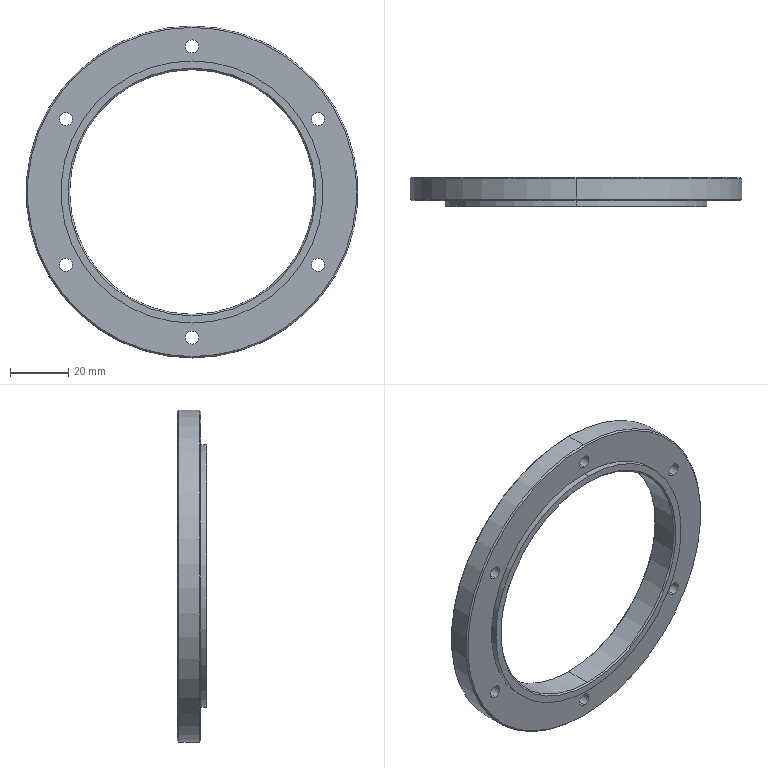Part | STEP file | 10-08 bearing seat cover plate lower | 1 solid | 47 faces | box 114 x 10 x 114 mm | volume 37218 mm3 | cylinder 30 | plane 9 | cone 8 | commonest cylinder face diameters 4.5 x12 8 x12 84 x2 90 x2 114 x2
STEP:
#1=CARTESIAN_POINT('',(0.,-0.5,-42.));
#2=VERTEX_POINT('',#1);
#3=CARTESIAN_POINT('',(0.,-0.5,42.));
#4=VERTEX_POINT('',#3);
#5=CARTESIAN_POINT('',(0.,-0.5,0.));
#6=DIRECTION('',(0.,1.,0.));
#7=DIRECTION('',(0.,0.,-1.));
#8=AXIS2_PLACEMENT_3D('',#5,#6,#7);
#9=CIRCLE('',#8,42.);
#10=EDGE_CURVE('',#2,#4,#9,.T.);
#11=ORIENTED_EDGE('',*,*,#10,.F.);
#12=CARTESIAN_POINT('',(0.,0.,-42.5));
#13=VERTEX_POINT('',#12);
#14=CARTESIAN_POINT('',(0.,-0.5,-42.));
#15=DIRECTION('',(0.,0.7071,-0.7071));
#16=VECTOR('',#15,1000.);
#17=LINE('',#14,#16);
#18=EDGE_CURVE('',#2,#13,#17,.T.);
#19=ORIENTED_EDGE('',*,*,#18,.T.);
#20=CARTESIAN_POINT('',(0.,0.,42.5));
#21=VERTEX_POINT('',#20);
#22=CARTESIAN_POINT('',(0.,0.,0.));
#23=DIRECTION('',(0.,-1.,0.));
#24=DIRECTION('',(0.,0.,-1.));
#25=AXIS2_PLACEMENT_3D('',#22,#23,#24);
#26=CIRCLE('',#25,42.5);
#27=EDGE_CURVE('',#21,#13,#26,.T.);
#28=ORIENTED_EDGE('',*,*,#27,.F.);
#29=CARTESIAN_POINT('',(0.,-0.5,42.));
#30=DIRECTION('',(0.,0.7071,0.7071));
#31=VECTOR('',#30,1000.);
#32=LINE('',#29,#31);
#33=EDGE_CURVE('',#4,#21,#32,.T.);
#34=ORIENTED_EDGE('',*,*,#33,.F.);
#35=EDGE_LOOP('',(#11,#19,#28,#34));
#36=FACE_OUTER_BOUND('',#35,.T.);
#37=CARTESIAN_POINT('',(0.,-0.5,0.));
#38=DIRECTION('',(0.,1.,0.));
#39=DIRECTION('',(0.,0.,1.));
#40=AXIS2_PLACEMENT_3D('',#37,#38,#39);
#41=CONICAL_SURFACE('',#40,42.,0.7854);
#42=ADVANCED_FACE('',(#36),#41,.F.);
#43=CARTESIAN_POINT('',(0.,0.,56.5));
#44=VERTEX_POINT('',#43);
#45=CARTESIAN_POINT('',(0.,0.,-56.5));
#46=VERTEX_POINT('',#45);
#47=CARTESIAN_POINT('',(0.,0.,0.));
#48=DIRECTION('',(0.,1.,0.));
#49=DIRECTION('',(0.,0.,-1.));
#50=AXIS2_PLACEMENT_3D('',#47,#48,#49);
#51=CIRCLE('',#50,56.5);
#52=EDGE_CURVE('',#44,#46,#51,.T.);
#53=ORIENTED_EDGE('',*,*,#52,.F.);
#54=CARTESIAN_POINT('',(0.,-0.5,57.));
#55=VERTEX_POINT('',#54);
#56=CARTESIAN_POINT('',(0.,0.,56.5));
#57=DIRECTION('',(0.,-0.7071,0.7071));
#58=VECTOR('',#57,1000.);
#59=LINE('',#56,#58);
#60=EDGE_CURVE('',#44,#55,#59,.T.);
#61=ORIENTED_EDGE('',*,*,#60,.T.);
#62=CARTESIAN_POINT('',(0.,-0.5,-57.));
#63=VERTEX_POINT('',#62);
#64=CARTESIAN_POINT('',(0.,-0.5,0.));
#65=DIRECTION('',(0.,-1.,0.));
#66=DIRECTION('',(0.,0.,-1.));
#67=AXIS2_PLACEMENT_3D('',#64,#65,#66);
#68=CIRCLE('',#67,57.);
#69=EDGE_CURVE('',#63,#55,#68,.T.);
#70=ORIENTED_EDGE('',*,*,#69,.F.);
#71=CARTESIAN_POINT('',(0.,0.,-56.5));
#72=DIRECTION('',(0.,-0.7071,-0.7071));
#73=VECTOR('',#72,1000.);
#74=LINE('',#71,#73);
#75=EDGE_CURVE('',#46,#63,#74,.T.);
#76=ORIENTED_EDGE('',*,*,#75,.F.);
#77=EDGE_LOOP('',(#53,#61,#70,#76));
#78=FACE_OUTER_BOUND('',#77,.T.);
#79=CARTESIAN_POINT('',(0.,0.,0.));
#80=DIRECTION('',(0.,-1.,0.));
#81=DIRECTION('',(0.,0.,-1.));
#82=AXIS2_PLACEMENT_3D('',#79,#80,#81);
#83=CONICAL_SURFACE('',#82,56.5,0.7854);
#84=ADVANCED_FACE('',(#78),#83,.T.);
#85=CARTESIAN_POINT('',(0.,-9.5,42.));
#86=VERTEX_POINT('',#85);
#87=CARTESIAN_POINT('',(0.,-9.5,-42.));
#88=VERTEX_POINT('',#87);
#89=CARTESIAN_POINT('',(0.,-9.5,0.));
#90=DIRECTION('',(0.,-1.,0.));
#91=DIRECTION('',(0.,0.,1.));
#92=AXIS2_PLACEMENT_3D('',#89,#90,#91);
#93=CIRCLE('',#92,42.);
#94=EDGE_CURVE('',#86,#88,#93,.T.);
#95=ORIENTED_EDGE('',*,*,#94,.F.);
#96=CARTESIAN_POINT('',(0.,-10.,42.5));
#97=VERTEX_POINT('',#96);
#98=CARTESIAN_POINT('',(0.,-10.,42.5));
#99=DIRECTION('',(0.,-0.7071,0.7071));
#100=VECTOR('',#99,1000.);
#101=LINE('',#98,#100);
#102=EDGE_CURVE('',#86,#97,#101,.T.);
#103=ORIENTED_EDGE('',*,*,#102,.T.);
#104=CARTESIAN_POINT('',(0.,-10.,-42.5));
#105=VERTEX_POINT('',#104);
#106=CARTESIAN_POINT('',(0.,-10.,0.));
#107=DIRECTION('',(0.,1.,0.));
#108=DIRECTION('',(0.,0.,1.));
#109=AXIS2_PLACEMENT_3D('',#106,#107,#108);
#110=CIRCLE('',#109,42.5);
#111=EDGE_CURVE('',#105,#97,#110,.T.);
#112=ORIENTED_EDGE('',*,*,#111,.F.);
#113=CARTESIAN_POINT('',(0.,-10.,-42.5));
#114=DIRECTION('',(0.,-0.7071,-0.7071));
#115=VECTOR('',#114,1000.);
#116=LINE('',#113,#115);
#117=EDGE_CURVE('',#88,#105,#116,.T.);
#118=ORIENTED_EDGE('',*,*,#117,.F.);
#119=EDGE_LOOP('',(#95,#103,#112,#118));
#120=FACE_OUTER_BOUND('',#119,.T.);
#121=CARTESIAN_POINT('',(0.,-10.,0.));
#122=DIRECTION('',(0.,-1.,0.));
#123=DIRECTION('',(0.,0.,-1.));
#124=AXIS2_PLACEMENT_3D('',#121,#122,#123);
#125=CONICAL_SURFACE('',#124,42.5,0.7854);
#126=ADVANCED_FACE('',(#120),#125,.F.);
#127=CARTESIAN_POINT('',(0.,-8.,-56.5));
#128=VERTEX_POINT('',#127);
#129=CARTESIAN_POINT('',(0.,-8.,56.5));
#130=VERTEX_POINT('',#129);
#131=CARTESIAN_POINT('',(0.,-8.,0.));
#132=DIRECTION('',(0.,-1.,0.));
#133=DIRECTION('',(0.,0.,1.));
#134=AXIS2_PLACEMENT_3D('',#131,#132,#133);
#135=CIRCLE('',#134,56.5);
#136=EDGE_CURVE('',#128,#130,#135,.T.);
#137=ORIENTED_EDGE('',*,*,#136,.F.);
#138=CARTESIAN_POINT('',(0.,-7.5,-57.));
#139=VERTEX_POINT('',#138);
#140=CARTESIAN_POINT('',(0.,-7.5,-57.));
#141=DIRECTION('',(0.,0.7071,-0.7071));
#142=VECTOR('',#141,1000.);
#143=LINE('',#140,#142);
#144=EDGE_CURVE('',#128,#139,#143,.T.);
#145=ORIENTED_EDGE('',*,*,#144,.T.);
#146=CARTESIAN_POINT('',(0.,-7.5,57.));
#147=VERTEX_POINT('',#146);
#148=CARTESIAN_POINT('',(0.,-7.5,0.));
#149=DIRECTION('',(0.,1.,0.));
#150=DIRECTION('',(0.,0.,1.));
#151=AXIS2_PLACEMENT_3D('',#148,#149,#150);
#152=CIRCLE('',#151,57.);
#153=EDGE_CURVE('',#147,#139,#152,.T.);
#154=ORIENTED_EDGE('',*,*,#153,.F.);
#155=CARTESIAN_POINT('',(0.,-7.5,57.));
#156=DIRECTION('',(0.,0.7071,0.7071));
#157=VECTOR('',#156,1000.);
#158=LINE('',#155,#157);
#159=EDGE_CURVE('',#130,#147,#158,.T.);
#160=ORIENTED_EDGE('',*,*,#159,.F.);
#161=EDGE_LOOP('',(#137,#145,#154,#160));
#162=FACE_OUTER_BOUND('',#161,.T.);
#163=CARTESIAN_POINT('',(0.,-7.5,0.));
#164=DIRECTION('',(0.,1.,0.));
#165=DIRECTION('',(0.,0.,1.));
#166=AXIS2_PLACEMENT_3D('',#163,#164,#165);
#167=CONICAL_SURFACE('',#166,57.,0.7854);
#168=ADVANCED_FACE('',(#162),#167,.T.);
#169=CARTESIAN_POINT('',(43.301,-4.,-29.));
#170=VERTEX_POINT('',#169);
#171=CARTESIAN_POINT('',(43.301,-4.,-21.));
#172=VERTEX_POINT('',#171);
#173=CARTESIAN_POINT('',(43.301,-4.,-25.));
#174=DIRECTION('',(0.,1.,0.));
#175=DIRECTION('',(0.,0.,1.));
#176=AXIS2_PLACEMENT_3D('',#173,#174,#175);
#177=CIRCLE('',#176,4.);
#178=EDGE_CURVE('',#170,#172,#177,.T.);
#179=ORIENTED_EDGE('',*,*,#178,.F.);
#180=CARTESIAN_POINT('',(43.301,0.,-29.));
#181=VERTEX_POINT('',#180);
#182=CARTESIAN_POINT('',(43.301,0.,-29.));
#183=DIRECTION('',(0.,1.,0.));
#184=VECTOR('',#183,1000.);
#185=LINE('',#182,#184);
#186=EDGE_CURVE('',#170,#181,#185,.T.);
#187=ORIENTED_EDGE('',*,*,#186,.T.);
#188=CARTESIAN_POINT('',(43.301,0.,-21.));
#189=VERTEX_POINT('',#188);
#190=CARTESIAN_POINT('',(43.301,0.,-25.));
#191=DIRECTION('',(0.,1.,0.));
#192=DIRECTION('',(0.,0.,1.));
#193=AXIS2_PLACEMENT_3D('',#190,#191,#192);
#194=CIRCLE('',#193,4.);
#195=EDGE_CURVE('',#181,#189,#194,.T.);
#196=ORIENTED_EDGE('',*,*,#195,.T.);
#197=CARTESIAN_POINT('',(43.301,0.,-21.));
#198=DIRECTION('',(0.,1.,0.));
#199=VECTOR('',#198,1000.);
#200=LINE('',#197,#199);
#201=EDGE_CURVE('',#172,#189,#200,.T.);
#202=ORIENTED_EDGE('',*,*,#201,.F.);
#203=EDGE_LOOP('',(#179,#187,#196,#202));
#204=FACE_OUTER_BOUND('',#203,.T.);
#205=CARTESIAN_POINT('',(43.301,0.,-25.));
#206=DIRECTION('',(0.,1.,0.));
#207=DIRECTION('',(0.,0.,1.));
#208=AXIS2_PLACEMENT_3D('',#205,#206,#207);
#209=CYLINDRICAL_SURFACE('',#208,4.);
#210=ADVANCED_FACE('',(#204),#209,.F.);
#211=CARTESIAN_POINT('',(43.301,-8.,-27.25));
#212=VERTEX_POINT('',#211);
#213=CARTESIAN_POINT('',(43.301,-8.,-22.75));
#214=VERTEX_POINT('',#213);
#215=CARTESIAN_POINT('',(43.301,-8.,-25.));
#216=DIRECTION('',(0.,1.,0.));
#217=DIRECTION('',(0.,0.,1.));
#218=AXIS2_PLACEMENT_3D('',#215,#216,#217);
#219=CIRCLE('',#218,2.25);
#220=EDGE_CURVE('',#212,#214,#219,.T.);
#221=ORIENTED_EDGE('',*,*,#220,.F.);
#222=CARTESIAN_POINT('',(43.301,-4.,-27.25));
#223=VERTEX_POINT('',#222);
#224=CARTESIAN_POINT('',(43.301,0.,-27.25));
#225=DIRECTION('',(0.,1.,0.));
#226=VECTOR('',#225,1000.);
#227=LINE('',#224,#226);
#228=EDGE_CURVE('',#212,#223,#227,.T.);
#229=ORIENTED_EDGE('',*,*,#228,.T.);
#230=CARTESIAN_POINT('',(43.301,-4.,-22.75));
#231=VERTEX_POINT('',#230);
#232=CARTESIAN_POINT('',(43.301,-4.,-25.));
#233=DIRECTION('',(0.,1.,0.));
#234=DIRECTION('',(0.,0.,1.));
#235=AXIS2_PLACEMENT_3D('',#232,#233,#234);
#236=CIRCLE('',#235,2.25);
#237=EDGE_CURVE('',#223,#231,#236,.T.);
#238=ORIENTED_EDGE('',*,*,#237,.T.);
#239=CARTESIAN_POINT('',(43.301,0.,-22.75));
#240=DIRECTION('',(0.,1.,0.));
#241=VECTOR('',#240,1000.);
#242=LINE('',#239,#241);
#243=EDGE_CURVE('',#214,#231,#242,.T.);
#244=ORIENTED_EDGE('',*,*,#243,.F.);
#245=EDGE_LOOP('',(#221,#229,#238,#244));
#246=FACE_OUTER_BOUND('',#245,.T.);
#247=CARTESIAN_POINT('',(43.301,0.,-25.));
#248=DIRECTION('',(0.,1.,0.));
#249=DIRECTION('',(0.,0.,1.));
#250=AXIS2_PLACEMENT_3D('',#247,#248,#249);
#251=CYLINDRICAL_SURFACE('',#250,2.25);
#252=ADVANCED_FACE('',(#246),#251,.F.);
#253=CARTESIAN_POINT('',(43.301,-4.,21.));
#254=VERTEX_POINT('',#253);
#255=CARTESIAN_POINT('',(43.301,-4.,29.));
#256=VERTEX_POINT('',#255);
#257=CARTESIAN_POINT('',(43.301,-4.,25.));
#258=DIRECTION('',(0.,1.,0.));
#259=DIRECTION('',(0.,0.,1.));
#260=AXIS2_PLACEMENT_3D('',#257,#258,#259);
#261=CIRCLE('',#260,4.);
#262=EDGE_CURVE('',#254,#256,#261,.T.);
#263=ORIENTED_EDGE('',*,*,#262,.F.);
#264=CARTESIAN_POINT('',(43.301,0.,21.));
#265=VERTEX_POINT('',#264);
#266=CARTESIAN_POINT('',(43.301,0.,21.));
#267=DIRECTION('',(0.,1.,0.));
#268=VECTOR('',#267,1000.);
#269=LINE('',#266,#268);
#270=EDGE_CURVE('',#254,#265,#269,.T.);
#271=ORIENTED_EDGE('',*,*,#270,.T.);
#272=CARTESIAN_POINT('',(43.301,0.,29.));
#273=VERTEX_POINT('',#272);
#274=CARTESIAN_POINT('',(43.301,0.,25.));
#275=DIRECTION('',(0.,1.,0.));
#276=DIRECTION('',(0.,0.,1.));
#277=AXIS2_PLACEMENT_3D('',#274,#275,#276);
#278=CIRCLE('',#277,4.);
#279=EDGE_CURVE('',#265,#273,#278,.T.);
#280=ORIENTED_EDGE('',*,*,#279,.T.);
#281=CARTESIAN_POINT('',(43.301,0.,29.));
#282=DIRECTION('',(0.,1.,0.));
#283=VECTOR('',#282,1000.);
#284=LINE('',#281,#283);
#285=EDGE_CURVE('',#256,#273,#284,.T.);
#286=ORIENTED_EDGE('',*,*,#285,.F.);
#287=EDGE_LOOP('',(#263,#271,#280,#286));
#288=FACE_OUTER_BOUND('',#287,.T.);
#289=CARTESIAN_POINT('',(43.301,0.,25.));
#290=DIRECTION('',(0.,1.,0.));
#291=DIRECTION('',(0.,0.,1.));
#292=AXIS2_PLACEMENT_3D('',#289,#290,#291);
#293=CYLINDRICAL_SURFACE('',#292,4.);
#294=ADVANCED_FACE('',(#288),#293,.F.);
#295=CARTESIAN_POINT('',(43.301,-8.,22.75));
#296=VERTEX_POINT('',#295);
#297=CARTESIAN_POINT('',(43.301,-8.,27.25));
#298=VERTEX_POINT('',#297);
#299=CARTESIAN_POINT('',(43.301,-8.,25.));
#300=DIRECTION('',(0.,1.,0.));
#301=DIRECTION('',(0.,0.,1.));
#302=AXIS2_PLACEMENT_3D('',#299,#300,#301);
#303=CIRCLE('',#302,2.25);
#304=EDGE_CURVE('',#296,#298,#303,.T.);
#305=ORIENTED_EDGE('',*,*,#304,.F.);
#306=CARTESIAN_POINT('',(43.301,-4.,22.75));
#307=VERTEX_POINT('',#306);
#308=CARTESIAN_POINT('',(43.301,0.,22.75));
#309=DIRECTION('',(0.,1.,0.));
#310=VECTOR('',#309,1000.);
#311=LINE('',#308,#310);
#312=EDGE_CURVE('',#296,#307,#311,.T.);
#313=ORIENTED_EDGE('',*,*,#312,.T.);
#314=CARTESIAN_POINT('',(43.301,-4.,27.25));
#315=VERTEX_POINT('',#314);
#316=CARTESIAN_POINT('',(43.301,-4.,25.));
#317=DIRECTION('',(0.,1.,0.));
#318=DIRECTION('',(0.,0.,1.));
#319=AXIS2_PLACEMENT_3D('',#316,#317,#318);
#320=CIRCLE('',#319,2.25);
#321=EDGE_CURVE('',#307,#315,#320,.T.);
#322=ORIENTED_EDGE('',*,*,#321,.T.);
#323=CARTESIAN_POINT('',(43.301,0.,27.25));
#324=DIRECTION('',(0.,1.,0.));
#325=VECTOR('',#324,1000.);
#326=LINE('',#323,#325);
#327=EDGE_CURVE('',#298,#315,#326,.T.);
#328=ORIENTED_EDGE('',*,*,#327,.F.);
#329=EDGE_LOOP('',(#305,#313,#322,#328));
#330=FACE_OUTER_BOUND('',#329,.T.);
#331=CARTESIAN_POINT('',(43.301,0.,25.));
#332=DIRECTION('',(0.,1.,0.));
#333=DIRECTION('',(0.,0.,1.));
#334=AXIS2_PLACEMENT_3D('',#331,#332,#333);
#335=CYLINDRICAL_SURFACE('',#334,2.25);
#336=ADVANCED_FACE('',(#330),#335,.F.);
#337=CARTESIAN_POINT('',(0.,-4.,46.));
#338=VERTEX_POINT('',#337);
#339=CARTESIAN_POINT('',(0.,-4.,54.));
#340=VERTEX_POINT('',#339);
#341=CARTESIAN_POINT('',(0.,-4.,50.));
#342=DIRECTION('',(0.,1.,0.));
#343=DIRECTION('',(0.,0.,1.));
#344=AXIS2_PLACEMENT_3D('',#341,#342,#343);
#345=CIRCLE('',#344,4.);
#346=EDGE_CURVE('',#338,#340,#345,.T.);
#347=ORIENTED_EDGE('',*,*,#346,.F.);
#348=CARTESIAN_POINT('',(0.,0.,46.));
#349=VERTEX_POINT('',#348);
#350=CARTESIAN_POINT('',(0.,0.,46.));
#351=DIRECTION('',(0.,1.,0.));
#352=VECTOR('',#351,1000.);
#353=LINE('',#350,#352);
#354=EDGE_CURVE('',#338,#349,#353,.T.);
#355=ORIENTED_EDGE('',*,*,#354,.T.);
#356=CARTESIAN_POINT('',(0.,0.,54.));
#357=VERTEX_POINT('',#356);
#358=CARTESIAN_POINT('',(0.,0.,50.));
#359=DIRECTION('',(0.,1.,0.));
#360=DIRECTION('',(0.,0.,1.));
#361=AXIS2_PLACEMENT_3D('',#358,#359,#360);
#362=CIRCLE('',#361,4.);
#363=EDGE_CURVE('',#349,#357,#362,.T.);
#364=ORIENTED_EDGE('',*,*,#363,.T.);
#365=CARTESIAN_POINT('',(0.,0.,54.));
#366=DIRECTION('',(0.,1.,0.));
#367=VECTOR('',#366,1000.);
#368=LINE('',#365,#367);
#369=EDGE_CURVE('',#340,#357,#368,.T.);
#370=ORIENTED_EDGE('',*,*,#369,.F.);
#371=EDGE_LOOP('',(#347,#355,#364,#370));
#372=FACE_OUTER_BOUND('',#371,.T.);
#373=CARTESIAN_POINT('',(0.,0.,50.));
#374=DIRECTION('',(0.,1.,0.));
#375=DIRECTION('',(0.,0.,1.));
#376=AXIS2_PLACEMENT_3D('',#373,#374,#375);
#377=CYLINDRICAL_SURFACE('',#376,4.);
#378=ADVANCED_FACE('',(#372),#377,.F.);
#379=CARTESIAN_POINT('',(0.,-8.,47.75));
#380=VERTEX_POINT('',#379);
#381=CARTESIAN_POINT('',(0.,-8.,52.25));
#382=VERTEX_POINT('',#381);
#383=CARTESIAN_POINT('',(0.,-8.,50.));
#384=DIRECTION('',(0.,1.,0.));
#385=DIRECTION('',(0.,0.,1.));
#386=AXIS2_PLACEMENT_3D('',#383,#384,#385);
#387=CIRCLE('',#386,2.25);
#388=EDGE_CURVE('',#380,#382,#387,.T.);
#389=ORIENTED_EDGE('',*,*,#388,.F.);
#390=CARTESIAN_POINT('',(0.,-4.,47.75));
#391=VERTEX_POINT('',#390);
#392=CARTESIAN_POINT('',(0.,0.,47.75));
#393=DIRECTION('',(0.,1.,0.));
#394=VECTOR('',#393,1000.);
#395=LINE('',#392,#394);
#396=EDGE_CURVE('',#380,#391,#395,.T.);
#397=ORIENTED_EDGE('',*,*,#396,.T.);
#398=CARTESIAN_POINT('',(0.,-4.,52.25));
#399=VERTEX_POINT('',#398);
#400=CARTESIAN_POINT('',(0.,-4.,50.));
#401=DIRECTION('',(0.,1.,0.));
#402=DIRECTION('',(0.,0.,1.));
#403=AXIS2_PLACEMENT_3D('',#400,#401,#402);
#404=CIRCLE('',#403,2.25);
#405=EDGE_CURVE('',#391,#399,#404,.T.);
#406=ORIENTED_EDGE('',*,*,#405,.T.);
#407=CARTESIAN_POINT('',(0.,0.,52.25));
#408=DIRECTION('',(0.,1.,0.));
#409=VECTOR('',#408,1000.);
#410=LINE('',#407,#409);
#411=EDGE_CURVE('',#382,#399,#410,.T.);
#412=ORIENTED_EDGE('',*,*,#411,.F.);
#413=EDGE_LOOP('',(#389,#397,#406,#412));
#414=FACE_OUTER_BOUND('',#413,.T.);
#415=CARTESIAN_POINT('',(0.,0.,50.));
#416=DIRECTION('',(0.,1.,0.));
#417=DIRECTION('',(0.,0.,1.));
#418=AXIS2_PLACEMENT_3D('',#415,#416,#417);
#419=CYLINDRICAL_SURFACE('',#418,2.25);
#420=ADVANCED_FACE('',(#414),#419,.F.);
#421=CARTESIAN_POINT('',(-43.301,-4.,21.));
#422=VERTEX_POINT('',#421);
#423=CARTESIAN_POINT('',(-43.301,-4.,29.));
#424=VERTEX_POINT('',#423);
#425=CARTESIAN_POINT('',(-43.301,-4.,25.));
#426=DIRECTION('',(0.,1.,0.));
#427=DIRECTION('',(0.,0.,1.));
#428=AXIS2_PLACEMENT_3D('',#425,#426,#427);
#429=CIRCLE('',#428,4.);
#430=EDGE_CURVE('',#422,#424,#429,.T.);
#431=ORIENTED_EDGE('',*,*,#430,.F.);
#432=CARTESIAN_POINT('',(-43.301,0.,21.));
#433=VERTEX_POINT('',#432);
#434=CARTESIAN_POINT('',(-43.301,0.,21.));
#435=DIRECTION('',(0.,1.,0.));
#436=VECTOR('',#435,1000.);
#437=LINE('',#434,#436);
#438=EDGE_CURVE('',#422,#433,#437,.T.);
#439=ORIENTED_EDGE('',*,*,#438,.T.);
#440=CARTESIAN_POINT('',(-43.301,0.,29.));
#441=VERTEX_POINT('',#440);
#442=CARTESIAN_POINT('',(-43.301,0.,25.));
#443=DIRECTION('',(0.,1.,0.));
#444=DIRECTION('',(0.,0.,1.));
#445=AXIS2_PLACEMENT_3D('',#442,#443,#444);
#446=CIRCLE('',#445,4.);
#447=EDGE_CURVE('',#433,#441,#446,.T.);
#448=ORIENTED_EDGE('',*,*,#447,.T.);
#449=CARTESIAN_POINT('',(-43.301,0.,29.));
#450=DIRECTION('',(0.,1.,0.));
#451=VECTOR('',#450,1000.);
#452=LINE('',#449,#451);
#453=EDGE_CURVE('',#424,#441,#452,.T.);
#454=ORIENTED_EDGE('',*,*,#453,.F.);
#455=EDGE_LOOP('',(#431,#439,#448,#454));
#456=FACE_OUTER_BOUND('',#455,.T.);
#457=CARTESIAN_POINT('',(-43.301,0.,25.));
#458=DIRECTION('',(0.,1.,0.));
#459=DIRECTION('',(0.,0.,1.));
#460=AXIS2_PLACEMENT_3D('',#457,#458,#459);
#461=CYLINDRICAL_SURFACE('',#460,4.);
#462=ADVANCED_FACE('',(#456),#461,.F.);
#463=CARTESIAN_POINT('',(-43.301,-8.,22.75));
#464=VERTEX_POINT('',#463);
#465=CARTESIAN_POINT('',(-43.301,-8.,27.25));
#466=VERTEX_POINT('',#465);
#467=CARTESIAN_POINT('',(-43.301,-8.,25.));
#468=DIRECTION('',(0.,1.,0.));
#469=DIRECTION('',(0.,0.,1.));
#470=AXIS2_PLACEMENT_3D('',#467,#468,#469);
#471=CIRCLE('',#470,2.25);
#472=EDGE_CURVE('',#464,#466,#471,.T.);
#473=ORIENTED_EDGE('',*,*,#472,.F.);
#474=CARTESIAN_POINT('',(-43.301,-4.,22.75));
#475=VERTEX_POINT('',#474);
#476=CARTESIAN_POINT('',(-43.301,0.,22.75));
#477=DIRECTION('',(0.,1.,0.));
#478=VECTOR('',#477,1000.);
#479=LINE('',#476,#478);
#480=EDGE_CURVE('',#464,#475,#479,.T.);
#481=ORIENTED_EDGE('',*,*,#480,.T.);
#482=CARTESIAN_POINT('',(-43.301,-4.,27.25));
#483=VERTEX_POINT('',#482);
#484=CARTESIAN_POINT('',(-43.301,-4.,25.));
#485=DIRECTION('',(0.,1.,0.));
#486=DIRECTION('',(0.,0.,1.));
#487=AXIS2_PLACEMENT_3D('',#484,#485,#486);
#488=CIRCLE('',#487,2.25);
#489=EDGE_CURVE('',#475,#483,#488,.T.);
#490=ORIENTED_EDGE('',*,*,#489,.T.);
#491=CARTESIAN_POINT('',(-43.301,0.,27.25));
#492=DIRECTION('',(0.,1.,0.));
#493=VECTOR('',#492,1000.);
#494=LINE('',#491,#493);
#495=EDGE_CURVE('',#466,#483,#494,.T.);
#496=ORIENTED_EDGE('',*,*,#495,.F.);
#497=EDGE_LOOP('',(#473,#481,#490,#496));
#498=FACE_OUTER_BOUND('',#497,.T.);
#499=CARTESIAN_POINT('',(-43.301,0.,25.));
#500=DIRECTION('',(0.,1.,0.));
#501=DIRECTION('',(0.,0.,1.));
#502=AXIS2_PLACEMENT_3D('',#499,#500,#501);
#503=CYLINDRICAL_SURFACE('',#502,2.25);
#504=ADVANCED_FACE('',(#498),#503,.F.);
#505=CARTESIAN_POINT('',(-43.301,-4.,-29.));
#506=VERTEX_POINT('',#505);
#507=CARTESIAN_POINT('',(-43.301,-4.,-21.));
#508=VERTEX_POINT('',#507);
#509=CARTESIAN_POINT('',(-43.301,-4.,-25.));
#510=DIRECTION('',(0.,1.,0.));
#511=DIRECTION('',(0.,0.,1.));
#512=AXIS2_PLACEMENT_3D('',#509,#510,#511);
#513=CIRCLE('',#512,4.);
#514=EDGE_CURVE('',#506,#508,#513,.T.);
#515=ORIENTED_EDGE('',*,*,#514,.F.);
#516=CARTESIAN_POINT('',(-43.301,0.,-29.));
#517=VERTEX_POINT('',#516);
#518=CARTESIAN_POINT('',(-43.301,0.,-29.));
#519=DIRECTION('',(0.,1.,0.));
#520=VECTOR('',#519,1000.);
#521=LINE('',#518,#520);
#522=EDGE_CURVE('',#506,#517,#521,.T.);
#523=ORIENTED_EDGE('',*,*,#522,.T.);
#524=CARTESIAN_POINT('',(-43.301,0.,-21.));
#525=VERTEX_POINT('',#524);
#526=CARTESIAN_POINT('',(-43.301,0.,-25.));
#527=DIRECTION('',(0.,1.,0.));
#528=DIRECTION('',(0.,0.,1.));
#529=AXIS2_PLACEMENT_3D('',#526,#527,#528);
#530=CIRCLE('',#529,4.);
#531=EDGE_CURVE('',#517,#525,#530,.T.);
#532=ORIENTED_EDGE('',*,*,#531,.T.);
#533=CARTESIAN_POINT('',(-43.301,0.,-21.));
#534=DIRECTION('',(0.,1.,0.));
#535=VECTOR('',#534,1000.);
#536=LINE('',#533,#535);
#537=EDGE_CURVE('',#508,#525,#536,.T.);
#538=ORIENTED_EDGE('',*,*,#537,.F.);
#539=EDGE_LOOP('',(#515,#523,#532,#538));
#540=FACE_OUTER_BOUND('',#539,.T.);
#541=CARTESIAN_POINT('',(-43.301,0.,-25.));
#542=DIRECTION('',(0.,1.,0.));
#543=DIRECTION('',(0.,0.,1.));
#544=AXIS2_PLACEMENT_3D('',#541,#542,#543);
#545=CYLINDRICAL_SURFACE('',#544,4.);
#546=ADVANCED_FACE('',(#540),#545,.F.);
#547=CARTESIAN_POINT('',(-43.301,-8.,-27.25));
#548=VERTEX_POINT('',#547);
#549=CARTESIAN_POINT('',(-43.301,-8.,-22.75));
#550=VERTEX_POINT('',#549);
#551=CARTESIAN_POINT('',(-43.301,-8.,-25.));
#552=DIRECTION('',(0.,1.,0.));
#553=DIRECTION('',(0.,0.,1.));
#554=AXIS2_PLACEMENT_3D('',#551,#552,#553);
#555=CIRCLE('',#554,2.25);
#556=EDGE_CURVE('',#548,#550,#555,.T.);
#557=ORIENTED_EDGE('',*,*,#556,.F.);
#558=CARTESIAN_POINT('',(-43.301,-4.,-27.25));
#559=VERTEX_POINT('',#558);
#560=CARTESIAN_POINT('',(-43.301,0.,-27.25));
#561=DIRECTION('',(0.,1.,0.));
#562=VECTOR('',#561,1000.);
#563=LINE('',#560,#562);
#564=EDGE_CURVE('',#548,#559,#563,.T.);
#565=ORIENTED_EDGE('',*,*,#564,.T.);
#566=CARTESIAN_POINT('',(-43.301,-4.,-22.75));
#567=VERTEX_POINT('',#566);
#568=CARTESIAN_POINT('',(-43.301,-4.,-25.));
#569=DIRECTION('',(0.,1.,0.));
#570=DIRECTION('',(0.,0.,1.));
#571=AXIS2_PLACEMENT_3D('',#568,#569,#570);
#572=CIRCLE('',#571,2.25);
#573=EDGE_CURVE('',#559,#567,#572,.T.);
#574=ORIENTED_EDGE('',*,*,#573,.T.);
#575=CARTESIAN_POINT('',(-43.301,0.,-22.75));
#576=DIRECTION('',(0.,1.,0.));
#577=VECTOR('',#576,1000.);
#578=LINE('',#575,#577);
#579=EDGE_CURVE('',#550,#567,#578,.T.);
#580=ORIENTED_EDGE('',*,*,#579,.F.);
#581=EDGE_LOOP('',(#557,#565,#574,#580));
#582=FACE_OUTER_BOUND('',#581,.T.);
#583=CARTESIAN_POINT('',(-43.301,0.,-25.));
#584=DIRECTION('',(0.,1.,0.));
#585=DIRECTION('',(0.,0.,1.));
#586=AXIS2_PLACEMENT_3D('',#583,#584,#585);
#587=CYLINDRICAL_SURFACE('',#586,2.25);
#588=ADVANCED_FACE('',(#582),#587,.F.);
#589=CARTESIAN_POINT('',(0.,-4.,-54.));
#590=VERTEX_POINT('',#589);
#591=CARTESIAN_POINT('',(0.,-4.,-46.));
#592=VERTEX_POINT('',#591);
#593=CARTESIAN_POINT('',(0.,-4.,-50.));
#594=DIRECTION('',(0.,1.,0.));
#595=DIRECTION('',(0.,0.,1.));
#596=AXIS2_PLACEMENT_3D('',#593,#594,#595);
#597=CIRCLE('',#596,4.);
#598=EDGE_CURVE('',#590,#592,#597,.T.);
#599=ORIENTED_EDGE('',*,*,#598,.F.);
#600=CARTESIAN_POINT('',(0.,0.,-54.));
#601=VERTEX_POINT('',#600);
#602=CARTESIAN_POINT('',(0.,0.,-54.));
#603=DIRECTION('',(0.,1.,0.));
#604=VECTOR('',#603,1000.);
#605=LINE('',#602,#604);
#606=EDGE_CURVE('',#590,#601,#605,.T.);
#607=ORIENTED_EDGE('',*,*,#606,.T.);
#608=CARTESIAN_POINT('',(0.,0.,-46.));
#609=VERTEX_POINT('',#608);
#610=CARTESIAN_POINT('',(0.,0.,-50.));
#611=DIRECTION('',(0.,1.,0.));
#612=DIRECTION('',(0.,0.,1.));
#613=AXIS2_PLACEMENT_3D('',#610,#611,#612);
#614=CIRCLE('',#613,4.);
#615=EDGE_CURVE('',#601,#609,#614,.T.);
#616=ORIENTED_EDGE('',*,*,#615,.T.);
#617=CARTESIAN_POINT('',(0.,0.,-46.));
#618=DIRECTION('',(0.,1.,0.));
#619=VECTOR('',#618,1000.);
#620=LINE('',#617,#619);
#621=EDGE_CURVE('',#592,#609,#620,.T.);
#622=ORIENTED_EDGE('',*,*,#621,.F.);
#623=EDGE_LOOP('',(#599,#607,#616,#622));
#624=FACE_OUTER_BOUND('',#623,.T.);
#625=CARTESIAN_POINT('',(0.,0.,-50.));
#626=DIRECTION('',(0.,1.,0.));
#627=DIRECTION('',(0.,0.,1.));
#628=AXIS2_PLACEMENT_3D('',#625,#626,#627);
#629=CYLINDRICAL_SURFACE('',#628,4.);
#630=ADVANCED_FACE('',(#624),#629,.F.);
#631=CARTESIAN_POINT('',(0.,-8.,-52.25));
#632=VERTEX_POINT('',#631);
#633=CARTESIAN_POINT('',(0.,-8.,-47.75));
#634=VERTEX_POINT('',#633);
#635=CARTESIAN_POINT('',(0.,-8.,-50.));
#636=DIRECTION('',(0.,1.,0.));
#637=DIRECTION('',(0.,0.,1.));
#638=AXIS2_PLACEMENT_3D('',#635,#636,#637);
#639=CIRCLE('',#638,2.25);
#640=EDGE_CURVE('',#632,#634,#639,.T.);
#641=ORIENTED_EDGE('',*,*,#640,.F.);
#642=CARTESIAN_POINT('',(0.,-4.,-52.25));
#643=VERTEX_POINT('',#642);
#644=CARTESIAN_POINT('',(0.,0.,-52.25));
#645=DIRECTION('',(0.,1.,0.));
#646=VECTOR('',#645,1000.);
#647=LINE('',#644,#646);
#648=EDGE_CURVE('',#632,#643,#647,.T.);
#649=ORIENTED_EDGE('',*,*,#648,.T.);
#650=CARTESIAN_POINT('',(0.,-4.,-47.75));
#651=VERTEX_POINT('',#650);
#652=CARTESIAN_POINT('',(0.,-4.,-50.));
#653=DIRECTION('',(0.,1.,0.));
#654=DIRECTION('',(0.,0.,1.));
#655=AXIS2_PLACEMENT_3D('',#652,#653,#654);
#656=CIRCLE('',#655,2.25);
#657=EDGE_CURVE('',#643,#651,#656,.T.);
#658=ORIENTED_EDGE('',*,*,#657,.T.);
#659=CARTESIAN_POINT('',(0.,0.,-47.75));
#660=DIRECTION('',(0.,1.,0.));
#661=VECTOR('',#660,1000.);
#662=LINE('',#659,#661);
#663=EDGE_CURVE('',#634,#651,#662,.T.);
#664=ORIENTED_EDGE('',*,*,#663,.F.);
#665=EDGE_LOOP('',(#641,#649,#658,#664));
#666=FACE_OUTER_BOUND('',#665,.T.);
#667=CARTESIAN_POINT('',(0.,0.,-50.));
#668=DIRECTION('',(0.,1.,0.));
#669=DIRECTION('',(0.,0.,1.));
#670=AXIS2_PLACEMENT_3D('',#667,#668,#669);
#671=CYLINDRICAL_SURFACE('',#670,2.25);
#672=ADVANCED_FACE('',(#666),#671,.F.);
#673=ORIENTED_EDGE('',*,*,#94,.T.);
#674=CARTESIAN_POINT('',(0.,0.,-42.));
#675=DIRECTION('',(0.,1.,0.));
#676=VECTOR('',#675,1000.);
#677=LINE('',#674,#676);
#678=EDGE_CURVE('',#88,#2,#677,.T.);
#679=ORIENTED_EDGE('',*,*,#678,.T.);
#680=ORIENTED_EDGE('',*,*,#10,.T.);
#681=CARTESIAN_POINT('',(0.,0.,42.));
#682=DIRECTION('',(0.,1.,0.));
#683=VECTOR('',#682,1000.);
#684=LINE('',#681,#683);
#685=EDGE_CURVE('',#86,#4,#684,.T.);
#686=ORIENTED_EDGE('',*,*,#685,.F.);
#687=EDGE_LOOP('',(#673,#679,#680,#686));
#688=FACE_OUTER_BOUND('',#687,.T.);
#689=CARTESIAN_POINT('',(0.,0.,0.));
#690=DIRECTION('',(0.,1.,0.));
#691=DIRECTION('',(0.,0.,1.));
#692=AXIS2_PLACEMENT_3D('',#689,#690,#691);
#693=CYLINDRICAL_SURFACE('',#692,42.);
#694=ADVANCED_FACE('',(#688),#693,.F.);
#695=CARTESIAN_POINT('',(0.,-10.,45.));
#696=VERTEX_POINT('',#695);
#697=CARTESIAN_POINT('',(0.,-10.,-45.));
#698=VERTEX_POINT('',#697);
#699=CARTESIAN_POINT('',(0.,-10.,0.));
#700=DIRECTION('',(0.,1.,0.));
#701=DIRECTION('',(0.,0.,1.));
#702=AXIS2_PLACEMENT_3D('',#699,#700,#701);
#703=CIRCLE('',#702,45.);
#704=EDGE_CURVE('',#696,#698,#703,.T.);
#705=ORIENTED_EDGE('',*,*,#704,.T.);
#706=CARTESIAN_POINT('',(0.,-8.,-45.));
#707=VERTEX_POINT('',#706);
#708=CARTESIAN_POINT('',(0.,0.,-45.));
#709=DIRECTION('',(0.,1.,0.));
#710=VECTOR('',#709,1000.);
#711=LINE('',#708,#710);
#712=EDGE_CURVE('',#698,#707,#711,.T.);
#713=ORIENTED_EDGE('',*,*,#712,.T.);
#714=CARTESIAN_POINT('',(0.,-8.,45.));
#715=VERTEX_POINT('',#714);
#716=CARTESIAN_POINT('',(0.,-8.,0.));
#717=DIRECTION('',(0.,1.,0.));
#718=DIRECTION('',(0.,0.,1.));
#719=AXIS2_PLACEMENT_3D('',#716,#717,#718);
#720=CIRCLE('',#719,45.);
#721=EDGE_CURVE('',#715,#707,#720,.T.);
#722=ORIENTED_EDGE('',*,*,#721,.F.);
#723=CARTESIAN_POINT('',(0.,0.,45.));
#724=DIRECTION('',(0.,1.,0.));
#725=VECTOR('',#724,1000.);
#726=LINE('',#723,#725);
#727=EDGE_CURVE('',#696,#715,#726,.T.);
#728=ORIENTED_EDGE('',*,*,#727,.F.);
#729=EDGE_LOOP('',(#705,#713,#722,#728));
#730=FACE_OUTER_BOUND('',#729,.T.);
#731=CARTESIAN_POINT('',(0.,0.,0.));
#732=DIRECTION('',(0.,1.,0.));
#733=DIRECTION('',(0.,0.,1.));
#734=AXIS2_PLACEMENT_3D('',#731,#732,#733);
#735=CYLINDRICAL_SURFACE('',#734,45.);
#736=ADVANCED_FACE('',(#730),#735,.T.);
#737=ORIENTED_EDGE('',*,*,#153,.T.);
#738=CARTESIAN_POINT('',(0.,0.,-57.));
#739=DIRECTION('',(0.,1.,0.));
#740=VECTOR('',#739,1000.);
#741=LINE('',#738,#740);
#742=EDGE_CURVE('',#139,#63,#741,.T.);
#743=ORIENTED_EDGE('',*,*,#742,.T.);
#744=ORIENTED_EDGE('',*,*,#69,.T.);
#745=CARTESIAN_POINT('',(0.,0.,57.));
#746=DIRECTION('',(0.,1.,0.));
#747=VECTOR('',#746,1000.);
#748=LINE('',#745,#747);
#749=EDGE_CURVE('',#147,#55,#748,.T.);
#750=ORIENTED_EDGE('',*,*,#749,.F.);
#751=EDGE_LOOP('',(#737,#743,#744,#750));
#752=FACE_OUTER_BOUND('',#751,.T.);
#753=CARTESIAN_POINT('',(0.,0.,0.));
#754=DIRECTION('',(0.,1.,0.));
#755=DIRECTION('',(0.,0.,1.));
#756=AXIS2_PLACEMENT_3D('',#753,#754,#755);
#757=CYLINDRICAL_SURFACE('',#756,57.);
#758=ADVANCED_FACE('',(#752),#757,.T.);
#759=ORIENTED_EDGE('',*,*,#742,.F.);
#760=CARTESIAN_POINT('',(0.,-7.5,0.));
#761=DIRECTION('',(0.,1.,0.));
#762=DIRECTION('',(0.,0.,1.));
#763=AXIS2_PLACEMENT_3D('',#760,#761,#762);
#764=CIRCLE('',#763,57.);
#765=EDGE_CURVE('',#139,#147,#764,.T.);
#766=ORIENTED_EDGE('',*,*,#765,.T.);
#767=ORIENTED_EDGE('',*,*,#749,.T.);
#768=CARTESIAN_POINT('',(0.,-0.5,0.));
#769=DIRECTION('',(0.,-1.,0.));
#770=DIRECTION('',(0.,0.,-1.));
#771=AXIS2_PLACEMENT_3D('',#768,#769,#770);
#772=CIRCLE('',#771,57.);
#773=EDGE_CURVE('',#55,#63,#772,.T.);
#774=ORIENTED_EDGE('',*,*,#773,.T.);
#775=EDGE_LOOP('',(#759,#766,#767,#774));
#776=FACE_OUTER_BOUND('',#775,.T.);
#777=CARTESIAN_POINT('',(0.,0.,0.));
#778=DIRECTION('',(0.,1.,0.));
#779=DIRECTION('',(0.,0.,1.));
#780=AXIS2_PLACEMENT_3D('',#777,#778,#779);
#781=CYLINDRICAL_SURFACE('',#780,57.);
#782=ADVANCED_FACE('',(#776),#781,.T.);
#783=CARTESIAN_POINT('',(0.,-8.,0.));
#784=DIRECTION('',(0.,-1.,0.));
#785=DIRECTION('',(0.,0.,1.));
#786=AXIS2_PLACEMENT_3D('',#783,#784,#785);
#787=CIRCLE('',#786,56.5);
#788=EDGE_CURVE('',#130,#128,#787,.T.);
#789=ORIENTED_EDGE('',*,*,#788,.T.);
#790=ORIENTED_EDGE('',*,*,#136,.T.);
#791=EDGE_LOOP('',(#789,#790));
#792=FACE_OUTER_BOUND('',#791,.T.);
#793=CARTESIAN_POINT('',(43.301,-8.,-25.));
#794=DIRECTION('',(0.,1.,0.));
#795=DIRECTION('',(0.,0.,1.));
#796=AXIS2_PLACEMENT_3D('',#793,#794,#795);
#797=CIRCLE('',#796,2.25);
#798=EDGE_CURVE('',#214,#212,#797,.T.);
#799=ORIENTED_EDGE('',*,*,#798,.T.);
#800=ORIENTED_EDGE('',*,*,#220,.T.);
#801=EDGE_LOOP('',(#799,#800));
#802=FACE_BOUND('',#801,.T.);
#803=CARTESIAN_POINT('',(43.301,-8.,25.));
#804=DIRECTION('',(0.,1.,0.));
#805=DIRECTION('',(0.,0.,1.));
#806=AXIS2_PLACEMENT_3D('',#803,#804,#805);
#807=CIRCLE('',#806,2.25);
#808=EDGE_CURVE('',#298,#296,#807,.T.);
#809=ORIENTED_EDGE('',*,*,#808,.T.);
#810=ORIENTED_EDGE('',*,*,#304,.T.);
#811=EDGE_LOOP('',(#809,#810));
#812=FACE_BOUND('',#811,.T.);
#813=CARTESIAN_POINT('',(0.,-8.,50.));
#814=DIRECTION('',(0.,1.,0.));
#815=DIRECTION('',(0.,0.,1.));
#816=AXIS2_PLACEMENT_3D('',#813,#814,#815);
#817=CIRCLE('',#816,2.25);
#818=EDGE_CURVE('',#382,#380,#817,.T.);
#819=ORIENTED_EDGE('',*,*,#818,.T.);
#820=ORIENTED_EDGE('',*,*,#388,.T.);
#821=EDGE_LOOP('',(#819,#820));
#822=FACE_BOUND('',#821,.T.);
#823=CARTESIAN_POINT('',(-43.301,-8.,25.));
#824=DIRECTION('',(0.,1.,0.));
#825=DIRECTION('',(0.,0.,1.));
#826=AXIS2_PLACEMENT_3D('',#823,#824,#825);
#827=CIRCLE('',#826,2.25);
#828=EDGE_CURVE('',#466,#464,#827,.T.);
#829=ORIENTED_EDGE('',*,*,#828,.T.);
#830=ORIENTED_EDGE('',*,*,#472,.T.);
#831=EDGE_LOOP('',(#829,#830));
#832=FACE_BOUND('',#831,.T.);
#833=CARTESIAN_POINT('',(-43.301,-8.,-25.));
#834=DIRECTION('',(0.,1.,0.));
#835=DIRECTION('',(0.,0.,1.));
#836=AXIS2_PLACEMENT_3D('',#833,#834,#835);
#837=CIRCLE('',#836,2.25);
#838=EDGE_CURVE('',#550,#548,#837,.T.);
#839=ORIENTED_EDGE('',*,*,#838,.T.);
#840=ORIENTED_EDGE('',*,*,#556,.T.);
#841=EDGE_LOOP('',(#839,#840));
#842=FACE_BOUND('',#841,.T.);
#843=CARTESIAN_POINT('',(0.,-8.,-50.));
#844=DIRECTION('',(0.,1.,0.));
#845=DIRECTION('',(0.,0.,1.));
#846=AXIS2_PLACEMENT_3D('',#843,#844,#845);
#847=CIRCLE('',#846,2.25);
#848=EDGE_CURVE('',#634,#632,#847,.T.);
#849=ORIENTED_EDGE('',*,*,#848,.T.);
#850=ORIENTED_EDGE('',*,*,#640,.T.);
#851=EDGE_LOOP('',(#849,#850));
#852=FACE_BOUND('',#851,.T.);
#853=ORIENTED_EDGE('',*,*,#721,.T.);
#854=CARTESIAN_POINT('',(0.,-8.,0.));
#855=DIRECTION('',(0.,1.,0.));
#856=DIRECTION('',(0.,0.,1.));
#857=AXIS2_PLACEMENT_3D('',#854,#855,#856);
#858=CIRCLE('',#857,45.);
#859=EDGE_CURVE('',#707,#715,#858,.T.);
#860=ORIENTED_EDGE('',*,*,#859,.T.);
#861=EDGE_LOOP('',(#853,#860));
#862=FACE_BOUND('',#861,.T.);
#863=CARTESIAN_POINT('',(57.,-8.,0.));
#864=DIRECTION('',(0.,1.,0.));
#865=DIRECTION('',(0.,0.,1.));
#866=AXIS2_PLACEMENT_3D('',#863,#864,#865);
#867=PLANE('',#866);
#868=ADVANCED_FACE('',(#792,#802,#812,#822,#832,#842,#852,#862),#867,.F.);
#869=ORIENTED_EDGE('',*,*,#712,.F.);
#870=CARTESIAN_POINT('',(0.,-10.,0.));
#871=DIRECTION('',(0.,1.,0.));
#872=DIRECTION('',(0.,0.,1.));
#873=AXIS2_PLACEMENT_3D('',#870,#871,#872);
#874=CIRCLE('',#873,45.);
#875=EDGE_CURVE('',#698,#696,#874,.T.);
#876=ORIENTED_EDGE('',*,*,#875,.T.);
#877=ORIENTED_EDGE('',*,*,#727,.T.);
#878=ORIENTED_EDGE('',*,*,#859,.F.);
#879=EDGE_LOOP('',(#869,#876,#877,#878));
#880=FACE_OUTER_BOUND('',#879,.T.);
#881=CARTESIAN_POINT('',(0.,0.,0.));
#882=DIRECTION('',(0.,1.,0.));
#883=DIRECTION('',(0.,0.,1.));
#884=AXIS2_PLACEMENT_3D('',#881,#882,#883);
#885=CYLINDRICAL_SURFACE('',#884,45.);
#886=ADVANCED_FACE('',(#880),#885,.T.);
#887=ORIENTED_EDGE('',*,*,#111,.T.);
#888=CARTESIAN_POINT('',(0.,-10.,0.));
#889=DIRECTION('',(0.,1.,0.));
#890=DIRECTION('',(0.,0.,1.));
#891=AXIS2_PLACEMENT_3D('',#888,#889,#890);
#892=CIRCLE('',#891,42.5);
#893=EDGE_CURVE('',#97,#105,#892,.T.);
#894=ORIENTED_EDGE('',*,*,#893,.T.);
#895=EDGE_LOOP('',(#887,#894));
#896=FACE_BOUND('',#895,.T.);
#897=ORIENTED_EDGE('',*,*,#704,.F.);
#898=ORIENTED_EDGE('',*,*,#875,.F.);
#899=EDGE_LOOP('',(#897,#898));
#900=FACE_OUTER_BOUND('',#899,.T.);
#901=CARTESIAN_POINT('',(45.,-10.,0.));
#902=DIRECTION('',(0.,1.,0.));
#903=DIRECTION('',(0.,0.,1.));
#904=AXIS2_PLACEMENT_3D('',#901,#902,#903);
#905=PLANE('',#904);
#906=ADVANCED_FACE('',(#896,#900),#905,.F.);
#907=ORIENTED_EDGE('',*,*,#678,.F.);
#908=CARTESIAN_POINT('',(0.,-9.5,0.));
#909=DIRECTION('',(0.,-1.,0.));
#910=DIRECTION('',(0.,0.,1.));
#911=AXIS2_PLACEMENT_3D('',#908,#909,#910);
#912=CIRCLE('',#911,42.);
#913=EDGE_CURVE('',#88,#86,#912,.T.);
#914=ORIENTED_EDGE('',*,*,#913,.T.);
#915=ORIENTED_EDGE('',*,*,#685,.T.);
#916=CARTESIAN_POINT('',(0.,-0.5,0.));
#917=DIRECTION('',(0.,1.,0.));
#918=DIRECTION('',(0.,0.,-1.));
#919=AXIS2_PLACEMENT_3D('',#916,#917,#918);
#920=CIRCLE('',#919,42.);
#921=EDGE_CURVE('',#4,#2,#920,.T.);
#922=ORIENTED_EDGE('',*,*,#921,.T.);
#923=EDGE_LOOP('',(#907,#914,#915,#922));
#924=FACE_OUTER_BOUND('',#923,.T.);
#925=CARTESIAN_POINT('',(0.,0.,0.));
#926=DIRECTION('',(0.,1.,0.));
#927=DIRECTION('',(0.,0.,1.));
#928=AXIS2_PLACEMENT_3D('',#925,#926,#927);
#929=CYLINDRICAL_SURFACE('',#928,42.);
#930=ADVANCED_FACE('',(#924),#929,.F.);
#931=CARTESIAN_POINT('',(0.,0.,0.));
#932=DIRECTION('',(0.,1.,0.));
#933=DIRECTION('',(0.,0.,-1.));
#934=AXIS2_PLACEMENT_3D('',#931,#932,#933);
#935=CIRCLE('',#934,56.5);
#936=EDGE_CURVE('',#46,#44,#935,.T.);
#937=ORIENTED_EDGE('',*,*,#936,.T.);
#938=ORIENTED_EDGE('',*,*,#52,.T.);
#939=EDGE_LOOP('',(#937,#938));
#940=FACE_OUTER_BOUND('',#939,.T.);
#941=ORIENTED_EDGE('',*,*,#27,.T.);
#942=CARTESIAN_POINT('',(0.,0.,0.));
#943=DIRECTION('',(0.,-1.,0.));
#944=DIRECTION('',(0.,0.,-1.));
#945=AXIS2_PLACEMENT_3D('',#942,#943,#944);
#946=CIRCLE('',#945,42.5);
#947=EDGE_CURVE('',#13,#21,#946,.T.);
#948=ORIENTED_EDGE('',*,*,#947,.T.);
#949=EDGE_LOOP('',(#941,#948));
#950=FACE_BOUND('',#949,.T.);
#951=CARTESIAN_POINT('',(43.301,0.,-25.));
#952=DIRECTION('',(0.,1.,0.));
#953=DIRECTION('',(0.,0.,1.));
#954=AXIS2_PLACEMENT_3D('',#951,#952,#953);
#955=CIRCLE('',#954,4.);
#956=EDGE_CURVE('',#189,#181,#955,.T.);
#957=ORIENTED_EDGE('',*,*,#956,.F.);
#958=ORIENTED_EDGE('',*,*,#195,.F.);
#959=EDGE_LOOP('',(#957,#958));
#960=FACE_BOUND('',#959,.T.);
#961=CARTESIAN_POINT('',(43.301,0.,25.));
#962=DIRECTION('',(0.,1.,0.));
#963=DIRECTION('',(0.,0.,1.));
#964=AXIS2_PLACEMENT_3D('',#961,#962,#963);
#965=CIRCLE('',#964,4.);
#966=EDGE_CURVE('',#273,#265,#965,.T.);
#967=ORIENTED_EDGE('',*,*,#966,.F.);
#968=ORIENTED_EDGE('',*,*,#279,.F.);
#969=EDGE_LOOP('',(#967,#968));
#970=FACE_BOUND('',#969,.T.);
#971=CARTESIAN_POINT('',(0.,0.,50.));
#972=DIRECTION('',(0.,1.,0.));
#973=DIRECTION('',(0.,0.,1.));
#974=AXIS2_PLACEMENT_3D('',#971,#972,#973);
#975=CIRCLE('',#974,4.);
#976=EDGE_CURVE('',#357,#349,#975,.T.);
#977=ORIENTED_EDGE('',*,*,#976,.F.);
#978=ORIENTED_EDGE('',*,*,#363,.F.);
#979=EDGE_LOOP('',(#977,#978));
#980=FACE_BOUND('',#979,.T.);
#981=CARTESIAN_POINT('',(-43.301,0.,25.));
#982=DIRECTION('',(0.,1.,0.));
#983=DIRECTION('',(0.,0.,1.));
#984=AXIS2_PLACEMENT_3D('',#981,#982,#983);
#985=CIRCLE('',#984,4.);
#986=EDGE_CURVE('',#441,#433,#985,.T.);
#987=ORIENTED_EDGE('',*,*,#986,.F.);
#988=ORIENTED_EDGE('',*,*,#447,.F.);
#989=EDGE_LOOP('',(#987,#988));
#990=FACE_BOUND('',#989,.T.);
#991=CARTESIAN_POINT('',(-43.301,0.,-25.));
#992=DIRECTION('',(0.,1.,0.));
#993=DIRECTION('',(0.,0.,1.));
#994=AXIS2_PLACEMENT_3D('',#991,#992,#993);
#995=CIRCLE('',#994,4.);
#996=EDGE_CURVE('',#525,#517,#995,.T.);
#997=ORIENTED_EDGE('',*,*,#996,.F.);
#998=ORIENTED_EDGE('',*,*,#531,.F.);
#999=EDGE_LOOP('',(#997,#998));
#1000=FACE_BOUND('',#999,.T.);
#1001=CARTESIAN_POINT('',(0.,0.,-50.));
#1002=DIRECTION('',(0.,1.,0.));
#1003=DIRECTION('',(0.,0.,1.));
#1004=AXIS2_PLACEMENT_3D('',#1001,#1002,#1003);
#1005=CIRCLE('',#1004,4.);
#1006=EDGE_CURVE('',#609,#601,#1005,.T.);
#1007=ORIENTED_EDGE('',*,*,#1006,.F.);
#1008=ORIENTED_EDGE('',*,*,#615,.F.);
#1009=EDGE_LOOP('',(#1007,#1008));
#1010=FACE_BOUND('',#1009,.T.);
#1011=CARTESIAN_POINT('',(57.,0.,0.));
#1012=DIRECTION('',(0.,-1.,0.));
#1013=DIRECTION('',(0.,0.,-1.));
#1014=AXIS2_PLACEMENT_3D('',#1011,#1012,#1013);
#1015=PLANE('',#1014);
#1016=ADVANCED_FACE('',(#940,#950,#960,#970,#980,#990,#1000,#1010),#1015,.F.);
#1017=ORIENTED_EDGE('',*,*,#648,.F.);
#1018=ORIENTED_EDGE('',*,*,#848,.F.);
#1019=ORIENTED_EDGE('',*,*,#663,.T.);
#1020=CARTESIAN_POINT('',(0.,-4.,-50.));
#1021=DIRECTION('',(0.,1.,0.));
#1022=DIRECTION('',(0.,0.,1.));
#1023=AXIS2_PLACEMENT_3D('',#1020,#1021,#1022);
#1024=CIRCLE('',#1023,2.25);
#1025=EDGE_CURVE('',#651,#643,#1024,.T.);
#1026=ORIENTED_EDGE('',*,*,#1025,.T.);
#1027=EDGE_LOOP('',(#1017,#1018,#1019,#1026));
#1028=FACE_OUTER_BOUND('',#1027,.T.);
#1029=CARTESIAN_POINT('',(0.,0.,-50.));
#1030=DIRECTION('',(0.,1.,0.));
#1031=DIRECTION('',(0.,0.,1.));
#1032=AXIS2_PLACEMENT_3D('',#1029,#1030,#1031);
#1033=CYLINDRICAL_SURFACE('',#1032,2.25);
#1034=ADVANCED_FACE('',(#1028),#1033,.F.);
#1035=ORIENTED_EDGE('',*,*,#1025,.F.);
#1036=ORIENTED_EDGE('',*,*,#657,.F.);
#1037=EDGE_LOOP('',(#1035,#1036));
#1038=FACE_BOUND('',#1037,.T.);
#1039=CARTESIAN_POINT('',(0.,-4.,-50.));
#1040=DIRECTION('',(0.,1.,0.));
#1041=DIRECTION('',(0.,0.,1.));
#1042=AXIS2_PLACEMENT_3D('',#1039,#1040,#1041);
#1043=CIRCLE('',#1042,4.);
#1044=EDGE_CURVE('',#592,#590,#1043,.T.);
#1045=ORIENTED_EDGE('',*,*,#1044,.T.);
#1046=ORIENTED_EDGE('',*,*,#598,.T.);
#1047=EDGE_LOOP('',(#1045,#1046));
#1048=FACE_OUTER_BOUND('',#1047,.T.);
#1049=CARTESIAN_POINT('',(2.25,-4.,-50.));
#1050=DIRECTION('',(0.,-1.,0.));
#1051=DIRECTION('',(0.,0.,-1.));
#1052=AXIS2_PLACEMENT_3D('',#1049,#1050,#1051);
#1053=PLANE('',#1052);
#1054=ADVANCED_FACE('',(#1038,#1048),#1053,.F.);
#1055=ORIENTED_EDGE('',*,*,#606,.F.);
#1056=ORIENTED_EDGE('',*,*,#1044,.F.);
#1057=ORIENTED_EDGE('',*,*,#621,.T.);
#1058=ORIENTED_EDGE('',*,*,#1006,.T.);
#1059=EDGE_LOOP('',(#1055,#1056,#1057,#1058));
#1060=FACE_OUTER_BOUND('',#1059,.T.);
#1061=CARTESIAN_POINT('',(0.,0.,-50.));
#1062=DIRECTION('',(0.,1.,0.));
#1063=DIRECTION('',(0.,0.,1.));
#1064=AXIS2_PLACEMENT_3D('',#1061,#1062,#1063);
#1065=CYLINDRICAL_SURFACE('',#1064,4.);
#1066=ADVANCED_FACE('',(#1060),#1065,.F.);
#1067=ORIENTED_EDGE('',*,*,#564,.F.);
#1068=ORIENTED_EDGE('',*,*,#838,.F.);
#1069=ORIENTED_EDGE('',*,*,#579,.T.);
#1070=CARTESIAN_POINT('',(-43.301,-4.,-25.));
#1071=DIRECTION('',(0.,1.,0.));
#1072=DIRECTION('',(0.,0.,1.));
#1073=AXIS2_PLACEMENT_3D('',#1070,#1071,#1072);
#1074=CIRCLE('',#1073,2.25);
#1075=EDGE_CURVE('',#567,#559,#1074,.T.);
#1076=ORIENTED_EDGE('',*,*,#1075,.T.);
#1077=EDGE_LOOP('',(#1067,#1068,#1069,#1076));
#1078=FACE_OUTER_BOUND('',#1077,.T.);
#1079=CARTESIAN_POINT('',(-43.301,0.,-25.));
#1080=DIRECTION('',(0.,1.,0.));
#1081=DIRECTION('',(0.,0.,1.));
#1082=AXIS2_PLACEMENT_3D('',#1079,#1080,#1081);
#1083=CYLINDRICAL_SURFACE('',#1082,2.25);
#1084=ADVANCED_FACE('',(#1078),#1083,.F.);
#1085=ORIENTED_EDGE('',*,*,#1075,.F.);
#1086=ORIENTED_EDGE('',*,*,#573,.F.);
#1087=EDGE_LOOP('',(#1085,#1086));
#1088=FACE_BOUND('',#1087,.T.);
#1089=CARTESIAN_POINT('',(-43.301,-4.,-25.));
#1090=DIRECTION('',(0.,1.,0.));
#1091=DIRECTION('',(0.,0.,1.));
#1092=AXIS2_PLACEMENT_3D('',#1089,#1090,#1091);
#1093=CIRCLE('',#1092,4.);
#1094=EDGE_CURVE('',#508,#506,#1093,.T.);
#1095=ORIENTED_EDGE('',*,*,#1094,.T.);
#1096=ORIENTED_EDGE('',*,*,#514,.T.);
#1097=EDGE_LOOP('',(#1095,#1096));
#1098=FACE_OUTER_BOUND('',#1097,.T.);
#1099=CARTESIAN_POINT('',(-41.051,-4.,-25.));
#1100=DIRECTION('',(0.,-1.,0.));
#1101=DIRECTION('',(0.,0.,-1.));
#1102=AXIS2_PLACEMENT_3D('',#1099,#1100,#1101);
#1103=PLANE('',#1102);
#1104=ADVANCED_FACE('',(#1088,#1098),#1103,.F.);
#1105=ORIENTED_EDGE('',*,*,#522,.F.);
#1106=ORIENTED_EDGE('',*,*,#1094,.F.);
#1107=ORIENTED_EDGE('',*,*,#537,.T.);
#1108=ORIENTED_EDGE('',*,*,#996,.T.);
#1109=EDGE_LOOP('',(#1105,#1106,#1107,#1108));
#1110=FACE_OUTER_BOUND('',#1109,.T.);
#1111=CARTESIAN_POINT('',(-43.301,0.,-25.));
#1112=DIRECTION('',(0.,1.,0.));
#1113=DIRECTION('',(0.,0.,1.));
#1114=AXIS2_PLACEMENT_3D('',#1111,#1112,#1113);
#1115=CYLINDRICAL_SURFACE('',#1114,4.);
#1116=ADVANCED_FACE('',(#1110),#1115,.F.);
#1117=ORIENTED_EDGE('',*,*,#480,.F.);
#1118=ORIENTED_EDGE('',*,*,#828,.F.);
#1119=ORIENTED_EDGE('',*,*,#495,.T.);
#1120=CARTESIAN_POINT('',(-43.301,-4.,25.));
#1121=DIRECTION('',(0.,1.,0.));
#1122=DIRECTION('',(0.,0.,1.));
#1123=AXIS2_PLACEMENT_3D('',#1120,#1121,#1122);
#1124=CIRCLE('',#1123,2.25);
#1125=EDGE_CURVE('',#483,#475,#1124,.T.);
#1126=ORIENTED_EDGE('',*,*,#1125,.T.);
#1127=EDGE_LOOP('',(#1117,#1118,#1119,#1126));
#1128=FACE_OUTER_BOUND('',#1127,.T.);
#1129=CARTESIAN_POINT('',(-43.301,0.,25.));
#1130=DIRECTION('',(0.,1.,0.));
#1131=DIRECTION('',(0.,0.,1.));
#1132=AXIS2_PLACEMENT_3D('',#1129,#1130,#1131);
#1133=CYLINDRICAL_SURFACE('',#1132,2.25);
#1134=ADVANCED_FACE('',(#1128),#1133,.F.);
#1135=ORIENTED_EDGE('',*,*,#1125,.F.);
#1136=ORIENTED_EDGE('',*,*,#489,.F.);
#1137=EDGE_LOOP('',(#1135,#1136));
#1138=FACE_BOUND('',#1137,.T.);
#1139=CARTESIAN_POINT('',(-43.301,-4.,25.));
#1140=DIRECTION('',(0.,1.,0.));
#1141=DIRECTION('',(0.,0.,1.));
#1142=AXIS2_PLACEMENT_3D('',#1139,#1140,#1141);
#1143=CIRCLE('',#1142,4.);
#1144=EDGE_CURVE('',#424,#422,#1143,.T.);
#1145=ORIENTED_EDGE('',*,*,#1144,.T.);
#1146=ORIENTED_EDGE('',*,*,#430,.T.);
#1147=EDGE_LOOP('',(#1145,#1146));
#1148=FACE_OUTER_BOUND('',#1147,.T.);
#1149=CARTESIAN_POINT('',(-41.051,-4.,25.));
#1150=DIRECTION('',(0.,-1.,0.));
#1151=DIRECTION('',(0.,0.,-1.));
#1152=AXIS2_PLACEMENT_3D('',#1149,#1150,#1151);
#1153=PLANE('',#1152);
#1154=ADVANCED_FACE('',(#1138,#1148),#1153,.F.);
#1155=ORIENTED_EDGE('',*,*,#438,.F.);
#1156=ORIENTED_EDGE('',*,*,#1144,.F.);
#1157=ORIENTED_EDGE('',*,*,#453,.T.);
#1158=ORIENTED_EDGE('',*,*,#986,.T.);
#1159=EDGE_LOOP('',(#1155,#1156,#1157,#1158));
#1160=FACE_OUTER_BOUND('',#1159,.T.);
#1161=CARTESIAN_POINT('',(-43.301,0.,25.));
#1162=DIRECTION('',(0.,1.,0.));
#1163=DIRECTION('',(0.,0.,1.));
#1164=AXIS2_PLACEMENT_3D('',#1161,#1162,#1163);
#1165=CYLINDRICAL_SURFACE('',#1164,4.);
#1166=ADVANCED_FACE('',(#1160),#1165,.F.);
#1167=ORIENTED_EDGE('',*,*,#396,.F.);
#1168=ORIENTED_EDGE('',*,*,#818,.F.);
#1169=ORIENTED_EDGE('',*,*,#411,.T.);
#1170=CARTESIAN_POINT('',(0.,-4.,50.));
#1171=DIRECTION('',(0.,1.,0.));
#1172=DIRECTION('',(0.,0.,1.));
#1173=AXIS2_PLACEMENT_3D('',#1170,#1171,#1172);
#1174=CIRCLE('',#1173,2.25);
#1175=EDGE_CURVE('',#399,#391,#1174,.T.);
#1176=ORIENTED_EDGE('',*,*,#1175,.T.);
#1177=EDGE_LOOP('',(#1167,#1168,#1169,#1176));
#1178=FACE_OUTER_BOUND('',#1177,.T.);
#1179=CARTESIAN_POINT('',(0.,0.,50.));
#1180=DIRECTION('',(0.,1.,0.));
#1181=DIRECTION('',(0.,0.,1.));
#1182=AXIS2_PLACEMENT_3D('',#1179,#1180,#1181);
#1183=CYLINDRICAL_SURFACE('',#1182,2.25);
#1184=ADVANCED_FACE('',(#1178),#1183,.F.);
#1185=ORIENTED_EDGE('',*,*,#1175,.F.);
#1186=ORIENTED_EDGE('',*,*,#405,.F.);
#1187=EDGE_LOOP('',(#1185,#1186));
#1188=FACE_BOUND('',#1187,.T.);
#1189=CARTESIAN_POINT('',(0.,-4.,50.));
#1190=DIRECTION('',(0.,1.,0.));
#1191=DIRECTION('',(0.,0.,1.));
#1192=AXIS2_PLACEMENT_3D('',#1189,#1190,#1191);
#1193=CIRCLE('',#1192,4.);
#1194=EDGE_CURVE('',#340,#338,#1193,.T.);
#1195=ORIENTED_EDGE('',*,*,#1194,.T.);
#1196=ORIENTED_EDGE('',*,*,#346,.T.);
#1197=EDGE_LOOP('',(#1195,#1196));
#1198=FACE_OUTER_BOUND('',#1197,.T.);
#1199=CARTESIAN_POINT('',(2.25,-4.,50.));
#1200=DIRECTION('',(0.,-1.,0.));
#1201=DIRECTION('',(0.,0.,-1.));
#1202=AXIS2_PLACEMENT_3D('',#1199,#1200,#1201);
#1203=PLANE('',#1202);
#1204=ADVANCED_FACE('',(#1188,#1198),#1203,.F.);
#1205=ORIENTED_EDGE('',*,*,#354,.F.);
#1206=ORIENTED_EDGE('',*,*,#1194,.F.);
#1207=ORIENTED_EDGE('',*,*,#369,.T.);
#1208=ORIENTED_EDGE('',*,*,#976,.T.);
#1209=EDGE_LOOP('',(#1205,#1206,#1207,#1208));
#1210=FACE_OUTER_BOUND('',#1209,.T.);
#1211=CARTESIAN_POINT('',(0.,0.,50.));
#1212=DIRECTION('',(0.,1.,0.));
#1213=DIRECTION('',(0.,0.,1.));
#1214=AXIS2_PLACEMENT_3D('',#1211,#1212,#1213);
#1215=CYLINDRICAL_SURFACE('',#1214,4.);
#1216=ADVANCED_FACE('',(#1210),#1215,.F.);
#1217=ORIENTED_EDGE('',*,*,#312,.F.);
#1218=ORIENTED_EDGE('',*,*,#808,.F.);
#1219=ORIENTED_EDGE('',*,*,#327,.T.);
#1220=CARTESIAN_POINT('',(43.301,-4.,25.));
#1221=DIRECTION('',(0.,1.,0.));
#1222=DIRECTION('',(0.,0.,1.));
#1223=AXIS2_PLACEMENT_3D('',#1220,#1221,#1222);
#1224=CIRCLE('',#1223,2.25);
#1225=EDGE_CURVE('',#315,#307,#1224,.T.);
#1226=ORIENTED_EDGE('',*,*,#1225,.T.);
#1227=EDGE_LOOP('',(#1217,#1218,#1219,#1226));
#1228=FACE_OUTER_BOUND('',#1227,.T.);
#1229=CARTESIAN_POINT('',(43.301,0.,25.));
#1230=DIRECTION('',(0.,1.,0.));
#1231=DIRECTION('',(0.,0.,1.));
#1232=AXIS2_PLACEMENT_3D('',#1229,#1230,#1231);
#1233=CYLINDRICAL_SURFACE('',#1232,2.25);
#1234=ADVANCED_FACE('',(#1228),#1233,.F.);
#1235=ORIENTED_EDGE('',*,*,#1225,.F.);
#1236=ORIENTED_EDGE('',*,*,#321,.F.);
#1237=EDGE_LOOP('',(#1235,#1236));
#1238=FACE_BOUND('',#1237,.T.);
#1239=CARTESIAN_POINT('',(43.301,-4.,25.));
#1240=DIRECTION('',(0.,1.,0.));
#1241=DIRECTION('',(0.,0.,1.));
#1242=AXIS2_PLACEMENT_3D('',#1239,#1240,#1241);
#1243=CIRCLE('',#1242,4.);
#1244=EDGE_CURVE('',#256,#254,#1243,.T.);
#1245=ORIENTED_EDGE('',*,*,#1244,.T.);
#1246=ORIENTED_EDGE('',*,*,#262,.T.);
#1247=EDGE_LOOP('',(#1245,#1246));
#1248=FACE_OUTER_BOUND('',#1247,.T.);
#1249=CARTESIAN_POINT('',(45.551,-4.,25.));
#1250=DIRECTION('',(0.,-1.,0.));
#1251=DIRECTION('',(0.,0.,-1.));
#1252=AXIS2_PLACEMENT_3D('',#1249,#1250,#1251);
#1253=PLANE('',#1252);
#1254=ADVANCED_FACE('',(#1238,#1248),#1253,.F.);
#1255=ORIENTED_EDGE('',*,*,#270,.F.);
#1256=ORIENTED_EDGE('',*,*,#1244,.F.);
#1257=ORIENTED_EDGE('',*,*,#285,.T.);
#1258=ORIENTED_EDGE('',*,*,#966,.T.);
#1259=EDGE_LOOP('',(#1255,#1256,#1257,#1258));
#1260=FACE_OUTER_BOUND('',#1259,.T.);
#1261=CARTESIAN_POINT('',(43.301,0.,25.));
#1262=DIRECTION('',(0.,1.,0.));
#1263=DIRECTION('',(0.,0.,1.));
#1264=AXIS2_PLACEMENT_3D('',#1261,#1262,#1263);
#1265=CYLINDRICAL_SURFACE('',#1264,4.);
#1266=ADVANCED_FACE('',(#1260),#1265,.F.);
#1267=ORIENTED_EDGE('',*,*,#228,.F.);
#1268=ORIENTED_EDGE('',*,*,#798,.F.);
#1269=ORIENTED_EDGE('',*,*,#243,.T.);
#1270=CARTESIAN_POINT('',(43.301,-4.,-25.));
#1271=DIRECTION('',(0.,1.,0.));
#1272=DIRECTION('',(0.,0.,1.));
#1273=AXIS2_PLACEMENT_3D('',#1270,#1271,#1272);
#1274=CIRCLE('',#1273,2.25);
#1275=EDGE_CURVE('',#231,#223,#1274,.T.);
#1276=ORIENTED_EDGE('',*,*,#1275,.T.);
#1277=EDGE_LOOP('',(#1267,#1268,#1269,#1276));
#1278=FACE_OUTER_BOUND('',#1277,.T.);
#1279=CARTESIAN_POINT('',(43.301,0.,-25.));
#1280=DIRECTION('',(0.,1.,0.));
#1281=DIRECTION('',(0.,0.,1.));
#1282=AXIS2_PLACEMENT_3D('',#1279,#1280,#1281);
#1283=CYLINDRICAL_SURFACE('',#1282,2.25);
#1284=ADVANCED_FACE('',(#1278),#1283,.F.);
#1285=ORIENTED_EDGE('',*,*,#1275,.F.);
#1286=ORIENTED_EDGE('',*,*,#237,.F.);
#1287=EDGE_LOOP('',(#1285,#1286));
#1288=FACE_BOUND('',#1287,.T.);
#1289=CARTESIAN_POINT('',(43.301,-4.,-25.));
#1290=DIRECTION('',(0.,1.,0.));
#1291=DIRECTION('',(0.,0.,1.));
#1292=AXIS2_PLACEMENT_3D('',#1289,#1290,#1291);
#1293=CIRCLE('',#1292,4.);
#1294=EDGE_CURVE('',#172,#170,#1293,.T.);
#1295=ORIENTED_EDGE('',*,*,#1294,.T.);
#1296=ORIENTED_EDGE('',*,*,#178,.T.);
#1297=EDGE_LOOP('',(#1295,#1296));
#1298=FACE_OUTER_BOUND('',#1297,.T.);
#1299=CARTESIAN_POINT('',(45.551,-4.,-25.));
#1300=DIRECTION('',(0.,-1.,0.));
#1301=DIRECTION('',(0.,0.,-1.));
#1302=AXIS2_PLACEMENT_3D('',#1299,#1300,#1301);
#1303=PLANE('',#1302);
#1304=ADVANCED_FACE('',(#1288,#1298),#1303,.F.);
#1305=ORIENTED_EDGE('',*,*,#186,.F.);
#1306=ORIENTED_EDGE('',*,*,#1294,.F.);
#1307=ORIENTED_EDGE('',*,*,#201,.T.);
#1308=ORIENTED_EDGE('',*,*,#956,.T.);
#1309=EDGE_LOOP('',(#1305,#1306,#1307,#1308));
#1310=FACE_OUTER_BOUND('',#1309,.T.);
#1311=CARTESIAN_POINT('',(43.301,0.,-25.));
#1312=DIRECTION('',(0.,1.,0.));
#1313=DIRECTION('',(0.,0.,1.));
#1314=AXIS2_PLACEMENT_3D('',#1311,#1312,#1313);
#1315=CYLINDRICAL_SURFACE('',#1314,4.);
#1316=ADVANCED_FACE('',(#1310),#1315,.F.);
#1317=ORIENTED_EDGE('',*,*,#144,.F.);
#1318=ORIENTED_EDGE('',*,*,#788,.F.);
#1319=ORIENTED_EDGE('',*,*,#159,.T.);
#1320=ORIENTED_EDGE('',*,*,#765,.F.);
#1321=EDGE_LOOP('',(#1317,#1318,#1319,#1320));
#1322=FACE_OUTER_BOUND('',#1321,.T.);
#1323=CARTESIAN_POINT('',(0.,-7.5,0.));
#1324=DIRECTION('',(0.,1.,0.));
#1325=DIRECTION('',(0.,0.,1.));
#1326=AXIS2_PLACEMENT_3D('',#1323,#1324,#1325);
#1327=CONICAL_SURFACE('',#1326,57.,0.7854);
#1328=ADVANCED_FACE('',(#1322),#1327,.T.);
#1329=ORIENTED_EDGE('',*,*,#102,.F.);
#1330=ORIENTED_EDGE('',*,*,#913,.F.);
#1331=ORIENTED_EDGE('',*,*,#117,.T.);
#1332=ORIENTED_EDGE('',*,*,#893,.F.);
#1333=EDGE_LOOP('',(#1329,#1330,#1331,#1332));
#1334=FACE_OUTER_BOUND('',#1333,.T.);
#1335=CARTESIAN_POINT('',(0.,-10.,0.));
#1336=DIRECTION('',(0.,-1.,0.));
#1337=DIRECTION('',(0.,0.,-1.));
#1338=AXIS2_PLACEMENT_3D('',#1335,#1336,#1337);
#1339=CONICAL_SURFACE('',#1338,42.5,0.7854);
#1340=ADVANCED_FACE('',(#1334),#1339,.F.);
#1341=ORIENTED_EDGE('',*,*,#60,.F.);
#1342=ORIENTED_EDGE('',*,*,#936,.F.);
#1343=ORIENTED_EDGE('',*,*,#75,.T.);
#1344=ORIENTED_EDGE('',*,*,#773,.F.);
#1345=EDGE_LOOP('',(#1341,#1342,#1343,#1344));
#1346=FACE_OUTER_BOUND('',#1345,.T.);
#1347=CARTESIAN_POINT('',(0.,0.,0.));
#1348=DIRECTION('',(0.,-1.,0.));
#1349=DIRECTION('',(0.,0.,-1.));
#1350=AXIS2_PLACEMENT_3D('',#1347,#1348,#1349);
#1351=CONICAL_SURFACE('',#1350,56.5,0.7854);
#1352=ADVANCED_FACE('',(#1346),#1351,.T.);
#1353=ORIENTED_EDGE('',*,*,#18,.F.);
#1354=ORIENTED_EDGE('',*,*,#921,.F.);
#1355=ORIENTED_EDGE('',*,*,#33,.T.);
#1356=ORIENTED_EDGE('',*,*,#947,.F.);
#1357=EDGE_LOOP('',(#1353,#1354,#1355,#1356));
#1358=FACE_OUTER_BOUND('',#1357,.T.);
#1359=CARTESIAN_POINT('',(0.,-0.5,0.));
#1360=DIRECTION('',(0.,1.,0.));
#1361=DIRECTION('',(0.,0.,1.));
#1362=AXIS2_PLACEMENT_3D('',#1359,#1360,#1361);
#1363=CONICAL_SURFACE('',#1362,42.,0.7854);
#1364=ADVANCED_FACE('',(#1358),#1363,.F.);
#1365=CLOSED_SHELL('',(#42,#84,#126,#168,#210,#252,#294,#336,#378,#420,#462,#504,#546,#588,#630,#672,#694,#736,#758,#782,#868,#886,#906,#930,#1016,#1034,#1054,#1066,#1084,#1104,#1116,#1134,#1154,#1166,#1184,#1204,#1216,#1234,#1254,#1266,#1284,#1304,#1316,#1328,#1340,#1352,#1364));
#1366=MANIFOLD_SOLID_BREP('',#1365);
#1367=CARTESIAN_POINT('',(0.,0.,0.));
#1368=DIRECTION('',(0.,0.,1.));
#1369=DIRECTION('',(1.,0.,0.));
#1370=AXIS2_PLACEMENT_3D('',#1367,#1368,#1369);
#1371=(LENGTH_UNIT()NAMED_UNIT(*)SI_UNIT(.MILLI.,.METRE.));
#1372=UNCERTAINTY_MEASURE_WITH_UNIT(LENGTH_MEASURE(0.00001),#1371,'','');
#1373=(NAMED_UNIT(*)PLANE_ANGLE_UNIT()SI_UNIT($,.RADIAN.));
#1374=(NAMED_UNIT(*)SI_UNIT($,.STERADIAN.)SOLID_ANGLE_UNIT());
#1375=(GEOMETRIC_REPRESENTATION_CONTEXT(3)GLOBAL_UNCERTAINTY_ASSIGNED_CONTEXT((#1372))GLOBAL_UNIT_ASSIGNED_CONTEXT((#1371,#1373,#1374))REPRESENTATION_CONTEXT('',''));
#1376=ADVANCED_BREP_SHAPE_REPRESENTATION('',(#1366,#1370),#1375);